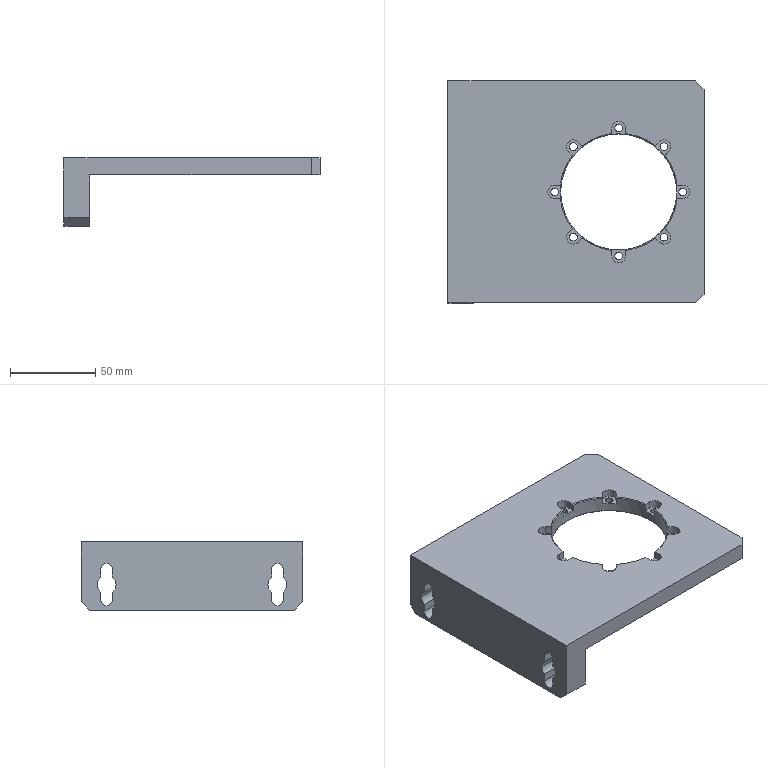NC program | NX | posted with a generic post | part box 150 x 130 x 40 mm
Lines 5777 to 5832 of 5832:
(PLANAR_MILL_COPY_COPY_COPY_COPY_COPY_COPY_1_COPY , TOOL : D6A45)
N11552 T01 M6
N11554 G54
N11556 G17 G0 G90 X-48.8 Y-33.095 B0. C0. S9500 M3
N11558 G43 Z30. H1
N11560 Z0.5
N11562 G94 G1 Z-1. F1250.
N11564 X-48.1 Y-32.691
N11566 G3 X-47.6 Y-31.825 R1.
N11568 G1 Y-29.45
N11570 G2 X-47.207 Y-28.655 R1.
N11572 G3 X-47.207 Y-21.345 R4.6
N11574 G2 X-47.6 Y-20.55 R1.
N11576 G1 Y-15.8
N11578 G3 X-50. Y-13.4 R2.4
N11580 X-52.4 Y-15.8 R2.4
N11582 G1 Y-20.55
N11584 G2 X-52.793 Y-21.345 R1.
N11586 G3 X-52.793 Y-28.655 R4.6
N11588 G2 X-52.4 Y-29.45 R1.
N11590 G1 Y-34.2
N11592 G3 X-50. Y-36.6 R2.4
N11594 X-47.6 Y-34.2 R2.4
N11596 G1 Y-31.825
N11598 G3 X-48.1 Y-30.959 R1.
N11600 G1 X-48.8 Y-30.555
N11602 Z0.5
N11604 G0 Z30.
N11606 X48.8
N11608 Z0.5
N11610 G1 Z-1.
N11612 X48.1 Y-30.959
N11614 G3 X47.6 Y-31.825 R1.
N11616 G1 Y-34.2
N11618 G3 X50. Y-36.6 R2.4
N11620 X52.4 Y-34.2 R2.4
N11622 G1 Y-29.45
N11624 G2 X52.793 Y-28.655 R1.
N11626 G3 X52.793 Y-21.345 R4.6
N11628 G2 X52.4 Y-20.55 R1.
N11630 G1 Y-15.8
N11632 G3 X50. Y-13.4 R2.4
N11634 X47.6 Y-15.8 R2.4
N11636 G1 Y-20.55
N11638 G2 X47.207 Y-21.345 R1.
N11640 G3 X47.207 Y-28.655 R4.6
N11642 G2 X47.6 Y-29.45 R1.
N11644 G1 Y-31.825
N11646 G3 X48.1 Y-32.691 R1.
N11648 G1 X48.8 Y-33.095
N11650 Z0.5
N11652 G0 Z30.
N11654 M5
N11656 M2